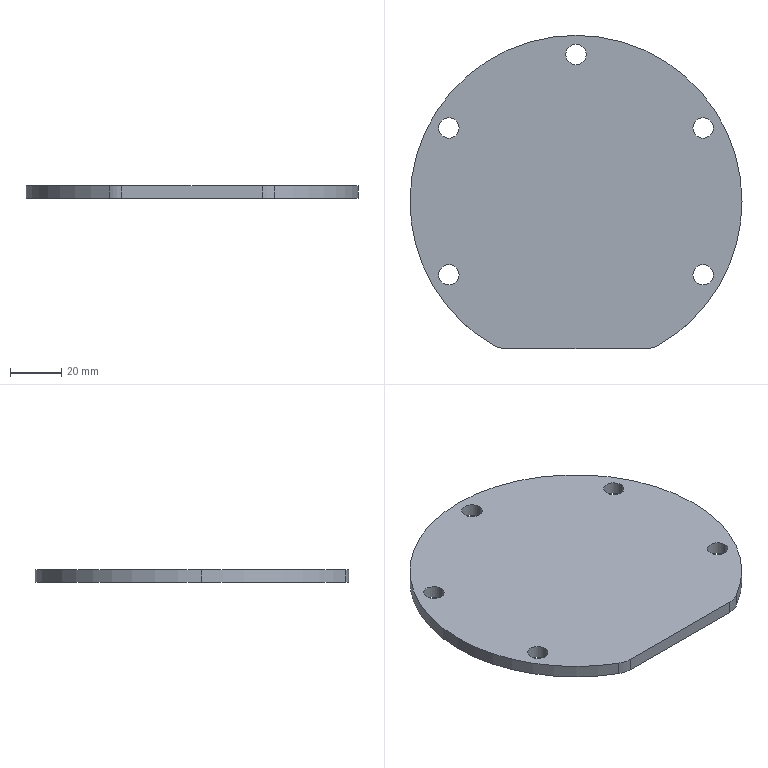Part | STEP file | VD-SYL0380DJ1006_1-3_VD-SYL0380 | 1 solid | 18 faces | box 130 x 122.663 x 5 mm | volume 63619 mm3 | cylinder 15 | plane 3 | commonest cylinder face diameters 8 x10 130 x3 20 x2
STEP:
#1=CARTESIAN_POINT('',(4.,57.5,0.));
#2=VERTEX_POINT('',#1);
#3=CARTESIAN_POINT('',(-4.,57.5,0.));
#4=VERTEX_POINT('',#3);
#5=CARTESIAN_POINT('',(0.,57.5,0.));
#6=DIRECTION('',(0.,0.,1.));
#7=DIRECTION('',(1.,0.,0.));
#8=AXIS2_PLACEMENT_3D('',#5,#6,#7);
#9=CIRCLE('',#8,4.);
#10=EDGE_CURVE('',#2,#4,#9,.T.);
#11=ORIENTED_EDGE('',*,*,#10,.F.);
#12=CARTESIAN_POINT('',(4.,57.5,5.));
#13=VERTEX_POINT('',#12);
#14=CARTESIAN_POINT('',(4.,57.5,5.));
#15=DIRECTION('',(0.,0.,-1.));
#16=VECTOR('',#15,1000.);
#17=LINE('',#14,#16);
#18=EDGE_CURVE('',#13,#2,#17,.T.);
#19=ORIENTED_EDGE('',*,*,#18,.F.);
#20=CARTESIAN_POINT('',(-4.,57.5,5.));
#21=VERTEX_POINT('',#20);
#22=CARTESIAN_POINT('',(0.,57.5,5.));
#23=DIRECTION('',(0.,0.,-1.));
#24=DIRECTION('',(-1.,0.,0.));
#25=AXIS2_PLACEMENT_3D('',#22,#23,#24);
#26=CIRCLE('',#25,4.);
#27=EDGE_CURVE('',#21,#13,#26,.T.);
#28=ORIENTED_EDGE('',*,*,#27,.F.);
#29=CARTESIAN_POINT('',(-4.,57.5,5.));
#30=DIRECTION('',(0.,0.,-1.));
#31=VECTOR('',#30,1000.);
#32=LINE('',#29,#31);
#33=EDGE_CURVE('',#21,#4,#32,.T.);
#34=ORIENTED_EDGE('',*,*,#33,.T.);
#35=EDGE_LOOP('',(#11,#19,#28,#34));
#36=FACE_OUTER_BOUND('',#35,.T.);
#37=CARTESIAN_POINT('',(0.,57.5,2.5));
#38=DIRECTION('',(0.,0.,1.));
#39=DIRECTION('',(1.,0.,0.));
#40=AXIS2_PLACEMENT_3D('',#37,#38,#39);
#41=CYLINDRICAL_SURFACE('',#40,4.);
#42=ADVANCED_FACE('',(#36),#41,.F.);
#43=ORIENTED_EDGE('',*,*,#33,.F.);
#44=CARTESIAN_POINT('',(0.,57.5,5.));
#45=DIRECTION('',(0.,0.,-1.));
#46=DIRECTION('',(1.,0.,0.));
#47=AXIS2_PLACEMENT_3D('',#44,#45,#46);
#48=CIRCLE('',#47,4.);
#49=EDGE_CURVE('',#13,#21,#48,.T.);
#50=ORIENTED_EDGE('',*,*,#49,.F.);
#51=ORIENTED_EDGE('',*,*,#18,.T.);
#52=CARTESIAN_POINT('',(0.,57.5,0.));
#53=DIRECTION('',(0.,0.,1.));
#54=DIRECTION('',(-1.,0.,0.));
#55=AXIS2_PLACEMENT_3D('',#52,#53,#54);
#56=CIRCLE('',#55,4.);
#57=EDGE_CURVE('',#4,#2,#56,.T.);
#58=ORIENTED_EDGE('',*,*,#57,.F.);
#59=EDGE_LOOP('',(#43,#50,#51,#58));
#60=FACE_OUTER_BOUND('',#59,.T.);
#61=CARTESIAN_POINT('',(0.,57.5,2.5));
#62=DIRECTION('',(0.,0.,1.));
#63=DIRECTION('',(1.,0.,0.));
#64=AXIS2_PLACEMENT_3D('',#61,#62,#63);
#65=CYLINDRICAL_SURFACE('',#64,4.);
#66=ADVANCED_FACE('',(#60),#65,.F.);
#67=CARTESIAN_POINT('',(-45.796,28.75,0.));
#68=VERTEX_POINT('',#67);
#69=CARTESIAN_POINT('',(-53.796,28.75,0.));
#70=VERTEX_POINT('',#69);
#71=CARTESIAN_POINT('',(-49.796,28.75,0.));
#72=DIRECTION('',(0.,0.,1.));
#73=DIRECTION('',(1.,0.,0.));
#74=AXIS2_PLACEMENT_3D('',#71,#72,#73);
#75=CIRCLE('',#74,4.);
#76=EDGE_CURVE('',#68,#70,#75,.T.);
#77=ORIENTED_EDGE('',*,*,#76,.F.);
#78=CARTESIAN_POINT('',(-45.796,28.75,5.));
#79=VERTEX_POINT('',#78);
#80=CARTESIAN_POINT('',(-45.796,28.75,5.));
#81=DIRECTION('',(0.,0.,-1.));
#82=VECTOR('',#81,1000.);
#83=LINE('',#80,#82);
#84=EDGE_CURVE('',#79,#68,#83,.T.);
#85=ORIENTED_EDGE('',*,*,#84,.F.);
#86=CARTESIAN_POINT('',(-53.796,28.75,5.));
#87=VERTEX_POINT('',#86);
#88=CARTESIAN_POINT('',(-49.796,28.75,5.));
#89=DIRECTION('',(0.,0.,-1.));
#90=DIRECTION('',(-1.,0.,0.));
#91=AXIS2_PLACEMENT_3D('',#88,#89,#90);
#92=CIRCLE('',#91,4.);
#93=EDGE_CURVE('',#87,#79,#92,.T.);
#94=ORIENTED_EDGE('',*,*,#93,.F.);
#95=CARTESIAN_POINT('',(-53.796,28.75,5.));
#96=DIRECTION('',(0.,0.,-1.));
#97=VECTOR('',#96,1000.);
#98=LINE('',#95,#97);
#99=EDGE_CURVE('',#87,#70,#98,.T.);
#100=ORIENTED_EDGE('',*,*,#99,.T.);
#101=EDGE_LOOP('',(#77,#85,#94,#100));
#102=FACE_OUTER_BOUND('',#101,.T.);
#103=CARTESIAN_POINT('',(-49.796,28.75,2.5));
#104=DIRECTION('',(0.,0.,1.));
#105=DIRECTION('',(1.,0.,0.));
#106=AXIS2_PLACEMENT_3D('',#103,#104,#105);
#107=CYLINDRICAL_SURFACE('',#106,4.);
#108=ADVANCED_FACE('',(#102),#107,.F.);
#109=ORIENTED_EDGE('',*,*,#99,.F.);
#110=CARTESIAN_POINT('',(-49.796,28.75,5.));
#111=DIRECTION('',(0.,0.,-1.));
#112=DIRECTION('',(1.,0.,0.));
#113=AXIS2_PLACEMENT_3D('',#110,#111,#112);
#114=CIRCLE('',#113,4.);
#115=EDGE_CURVE('',#79,#87,#114,.T.);
#116=ORIENTED_EDGE('',*,*,#115,.F.);
#117=ORIENTED_EDGE('',*,*,#84,.T.);
#118=CARTESIAN_POINT('',(-49.796,28.75,0.));
#119=DIRECTION('',(0.,0.,1.));
#120=DIRECTION('',(-1.,0.,0.));
#121=AXIS2_PLACEMENT_3D('',#118,#119,#120);
#122=CIRCLE('',#121,4.);
#123=EDGE_CURVE('',#70,#68,#122,.T.);
#124=ORIENTED_EDGE('',*,*,#123,.F.);
#125=EDGE_LOOP('',(#109,#116,#117,#124));
#126=FACE_OUTER_BOUND('',#125,.T.);
#127=CARTESIAN_POINT('',(-49.796,28.75,2.5));
#128=DIRECTION('',(0.,0.,1.));
#129=DIRECTION('',(1.,0.,0.));
#130=AXIS2_PLACEMENT_3D('',#127,#128,#129);
#131=CYLINDRICAL_SURFACE('',#130,4.);
#132=ADVANCED_FACE('',(#126),#131,.F.);
#133=CARTESIAN_POINT('',(-45.796,-28.75,0.));
#134=VERTEX_POINT('',#133);
#135=CARTESIAN_POINT('',(-53.796,-28.75,0.));
#136=VERTEX_POINT('',#135);
#137=CARTESIAN_POINT('',(-49.796,-28.75,0.));
#138=DIRECTION('',(0.,0.,1.));
#139=DIRECTION('',(1.,0.,0.));
#140=AXIS2_PLACEMENT_3D('',#137,#138,#139);
#141=CIRCLE('',#140,4.);
#142=EDGE_CURVE('',#134,#136,#141,.T.);
#143=ORIENTED_EDGE('',*,*,#142,.F.);
#144=CARTESIAN_POINT('',(-45.796,-28.75,5.));
#145=VERTEX_POINT('',#144);
#146=CARTESIAN_POINT('',(-45.796,-28.75,5.));
#147=DIRECTION('',(0.,0.,-1.));
#148=VECTOR('',#147,1000.);
#149=LINE('',#146,#148);
#150=EDGE_CURVE('',#145,#134,#149,.T.);
#151=ORIENTED_EDGE('',*,*,#150,.F.);
#152=CARTESIAN_POINT('',(-53.796,-28.75,5.));
#153=VERTEX_POINT('',#152);
#154=CARTESIAN_POINT('',(-49.796,-28.75,5.));
#155=DIRECTION('',(0.,0.,-1.));
#156=DIRECTION('',(-1.,0.,0.));
#157=AXIS2_PLACEMENT_3D('',#154,#155,#156);
#158=CIRCLE('',#157,4.);
#159=EDGE_CURVE('',#153,#145,#158,.T.);
#160=ORIENTED_EDGE('',*,*,#159,.F.);
#161=CARTESIAN_POINT('',(-53.796,-28.75,5.));
#162=DIRECTION('',(0.,0.,-1.));
#163=VECTOR('',#162,1000.);
#164=LINE('',#161,#163);
#165=EDGE_CURVE('',#153,#136,#164,.T.);
#166=ORIENTED_EDGE('',*,*,#165,.T.);
#167=EDGE_LOOP('',(#143,#151,#160,#166));
#168=FACE_OUTER_BOUND('',#167,.T.);
#169=CARTESIAN_POINT('',(-49.796,-28.75,2.5));
#170=DIRECTION('',(0.,0.,1.));
#171=DIRECTION('',(1.,0.,0.));
#172=AXIS2_PLACEMENT_3D('',#169,#170,#171);
#173=CYLINDRICAL_SURFACE('',#172,4.);
#174=ADVANCED_FACE('',(#168),#173,.F.);
#175=ORIENTED_EDGE('',*,*,#165,.F.);
#176=CARTESIAN_POINT('',(-49.796,-28.75,5.));
#177=DIRECTION('',(0.,0.,-1.));
#178=DIRECTION('',(1.,0.,0.));
#179=AXIS2_PLACEMENT_3D('',#176,#177,#178);
#180=CIRCLE('',#179,4.);
#181=EDGE_CURVE('',#145,#153,#180,.T.);
#182=ORIENTED_EDGE('',*,*,#181,.F.);
#183=ORIENTED_EDGE('',*,*,#150,.T.);
#184=CARTESIAN_POINT('',(-49.796,-28.75,0.));
#185=DIRECTION('',(0.,0.,1.));
#186=DIRECTION('',(-1.,0.,0.));
#187=AXIS2_PLACEMENT_3D('',#184,#185,#186);
#188=CIRCLE('',#187,4.);
#189=EDGE_CURVE('',#136,#134,#188,.T.);
#190=ORIENTED_EDGE('',*,*,#189,.F.);
#191=EDGE_LOOP('',(#175,#182,#183,#190));
#192=FACE_OUTER_BOUND('',#191,.T.);
#193=CARTESIAN_POINT('',(-49.796,-28.75,2.5));
#194=DIRECTION('',(0.,0.,1.));
#195=DIRECTION('',(1.,0.,0.));
#196=AXIS2_PLACEMENT_3D('',#193,#194,#195);
#197=CYLINDRICAL_SURFACE('',#196,4.);
#198=ADVANCED_FACE('',(#192),#197,.F.);
#199=CARTESIAN_POINT('',(53.796,-28.75,0.));
#200=VERTEX_POINT('',#199);
#201=CARTESIAN_POINT('',(45.796,-28.75,0.));
#202=VERTEX_POINT('',#201);
#203=CARTESIAN_POINT('',(49.796,-28.75,0.));
#204=DIRECTION('',(0.,0.,1.));
#205=DIRECTION('',(1.,0.,0.));
#206=AXIS2_PLACEMENT_3D('',#203,#204,#205);
#207=CIRCLE('',#206,4.);
#208=EDGE_CURVE('',#200,#202,#207,.T.);
#209=ORIENTED_EDGE('',*,*,#208,.F.);
#210=CARTESIAN_POINT('',(53.796,-28.75,5.));
#211=VERTEX_POINT('',#210);
#212=CARTESIAN_POINT('',(53.796,-28.75,5.));
#213=DIRECTION('',(0.,0.,-1.));
#214=VECTOR('',#213,1000.);
#215=LINE('',#212,#214);
#216=EDGE_CURVE('',#211,#200,#215,.T.);
#217=ORIENTED_EDGE('',*,*,#216,.F.);
#218=CARTESIAN_POINT('',(45.796,-28.75,5.));
#219=VERTEX_POINT('',#218);
#220=CARTESIAN_POINT('',(49.796,-28.75,5.));
#221=DIRECTION('',(0.,0.,-1.));
#222=DIRECTION('',(-1.,0.,0.));
#223=AXIS2_PLACEMENT_3D('',#220,#221,#222);
#224=CIRCLE('',#223,4.);
#225=EDGE_CURVE('',#219,#211,#224,.T.);
#226=ORIENTED_EDGE('',*,*,#225,.F.);
#227=CARTESIAN_POINT('',(45.796,-28.75,5.));
#228=DIRECTION('',(0.,0.,-1.));
#229=VECTOR('',#228,1000.);
#230=LINE('',#227,#229);
#231=EDGE_CURVE('',#219,#202,#230,.T.);
#232=ORIENTED_EDGE('',*,*,#231,.T.);
#233=EDGE_LOOP('',(#209,#217,#226,#232));
#234=FACE_OUTER_BOUND('',#233,.T.);
#235=CARTESIAN_POINT('',(49.796,-28.75,2.5));
#236=DIRECTION('',(0.,0.,1.));
#237=DIRECTION('',(1.,0.,0.));
#238=AXIS2_PLACEMENT_3D('',#235,#236,#237);
#239=CYLINDRICAL_SURFACE('',#238,4.);
#240=ADVANCED_FACE('',(#234),#239,.F.);
#241=ORIENTED_EDGE('',*,*,#231,.F.);
#242=CARTESIAN_POINT('',(49.796,-28.75,5.));
#243=DIRECTION('',(0.,0.,-1.));
#244=DIRECTION('',(1.,0.,0.));
#245=AXIS2_PLACEMENT_3D('',#242,#243,#244);
#246=CIRCLE('',#245,4.);
#247=EDGE_CURVE('',#211,#219,#246,.T.);
#248=ORIENTED_EDGE('',*,*,#247,.F.);
#249=ORIENTED_EDGE('',*,*,#216,.T.);
#250=CARTESIAN_POINT('',(49.796,-28.75,0.));
#251=DIRECTION('',(0.,0.,1.));
#252=DIRECTION('',(-1.,0.,0.));
#253=AXIS2_PLACEMENT_3D('',#250,#251,#252);
#254=CIRCLE('',#253,4.);
#255=EDGE_CURVE('',#202,#200,#254,.T.);
#256=ORIENTED_EDGE('',*,*,#255,.F.);
#257=EDGE_LOOP('',(#241,#248,#249,#256));
#258=FACE_OUTER_BOUND('',#257,.T.);
#259=CARTESIAN_POINT('',(49.796,-28.75,2.5));
#260=DIRECTION('',(0.,0.,1.));
#261=DIRECTION('',(1.,0.,0.));
#262=AXIS2_PLACEMENT_3D('',#259,#260,#261);
#263=CYLINDRICAL_SURFACE('',#262,4.);
#264=ADVANCED_FACE('',(#258),#263,.F.);
#265=CARTESIAN_POINT('',(53.796,28.75,0.));
#266=VERTEX_POINT('',#265);
#267=CARTESIAN_POINT('',(45.796,28.75,0.));
#268=VERTEX_POINT('',#267);
#269=CARTESIAN_POINT('',(49.796,28.75,0.));
#270=DIRECTION('',(0.,0.,1.));
#271=DIRECTION('',(1.,0.,0.));
#272=AXIS2_PLACEMENT_3D('',#269,#270,#271);
#273=CIRCLE('',#272,4.);
#274=EDGE_CURVE('',#266,#268,#273,.T.);
#275=ORIENTED_EDGE('',*,*,#274,.F.);
#276=CARTESIAN_POINT('',(53.796,28.75,5.));
#277=VERTEX_POINT('',#276);
#278=CARTESIAN_POINT('',(53.796,28.75,5.));
#279=DIRECTION('',(0.,0.,-1.));
#280=VECTOR('',#279,1000.);
#281=LINE('',#278,#280);
#282=EDGE_CURVE('',#277,#266,#281,.T.);
#283=ORIENTED_EDGE('',*,*,#282,.F.);
#284=CARTESIAN_POINT('',(45.796,28.75,5.));
#285=VERTEX_POINT('',#284);
#286=CARTESIAN_POINT('',(49.796,28.75,5.));
#287=DIRECTION('',(0.,0.,-1.));
#288=DIRECTION('',(-1.,0.,0.));
#289=AXIS2_PLACEMENT_3D('',#286,#287,#288);
#290=CIRCLE('',#289,4.);
#291=EDGE_CURVE('',#285,#277,#290,.T.);
#292=ORIENTED_EDGE('',*,*,#291,.F.);
#293=CARTESIAN_POINT('',(45.796,28.75,5.));
#294=DIRECTION('',(0.,0.,-1.));
#295=VECTOR('',#294,1000.);
#296=LINE('',#293,#295);
#297=EDGE_CURVE('',#285,#268,#296,.T.);
#298=ORIENTED_EDGE('',*,*,#297,.T.);
#299=EDGE_LOOP('',(#275,#283,#292,#298));
#300=FACE_OUTER_BOUND('',#299,.T.);
#301=CARTESIAN_POINT('',(49.796,28.75,2.5));
#302=DIRECTION('',(0.,0.,1.));
#303=DIRECTION('',(1.,0.,0.));
#304=AXIS2_PLACEMENT_3D('',#301,#302,#303);
#305=CYLINDRICAL_SURFACE('',#304,4.);
#306=ADVANCED_FACE('',(#300),#305,.F.);
#307=ORIENTED_EDGE('',*,*,#297,.F.);
#308=CARTESIAN_POINT('',(49.796,28.75,5.));
#309=DIRECTION('',(0.,0.,-1.));
#310=DIRECTION('',(1.,0.,0.));
#311=AXIS2_PLACEMENT_3D('',#308,#309,#310);
#312=CIRCLE('',#311,4.);
#313=EDGE_CURVE('',#277,#285,#312,.T.);
#314=ORIENTED_EDGE('',*,*,#313,.F.);
#315=ORIENTED_EDGE('',*,*,#282,.T.);
#316=CARTESIAN_POINT('',(49.796,28.75,0.));
#317=DIRECTION('',(0.,0.,1.));
#318=DIRECTION('',(-1.,0.,0.));
#319=AXIS2_PLACEMENT_3D('',#316,#317,#318);
#320=CIRCLE('',#319,4.);
#321=EDGE_CURVE('',#268,#266,#320,.T.);
#322=ORIENTED_EDGE('',*,*,#321,.F.);
#323=EDGE_LOOP('',(#307,#314,#315,#322));
#324=FACE_OUTER_BOUND('',#323,.T.);
#325=CARTESIAN_POINT('',(49.796,28.75,2.5));
#326=DIRECTION('',(0.,0.,1.));
#327=DIRECTION('',(1.,0.,0.));
#328=AXIS2_PLACEMENT_3D('',#325,#326,#327);
#329=CYLINDRICAL_SURFACE('',#328,4.);
#330=ADVANCED_FACE('',(#324),#329,.F.);
#331=CARTESIAN_POINT('',(-27.446,-57.663,0.));
#332=VERTEX_POINT('',#331);
#333=CARTESIAN_POINT('',(-32.436,-56.329,0.));
#334=VERTEX_POINT('',#333);
#335=CARTESIAN_POINT('',(-27.446,-47.663,0.));
#336=DIRECTION('',(0.,0.,-1.));
#337=DIRECTION('',(0.,-1.,0.));
#338=AXIS2_PLACEMENT_3D('',#335,#336,#337);
#339=CIRCLE('',#338,10.);
#340=EDGE_CURVE('',#332,#334,#339,.T.);
#341=ORIENTED_EDGE('',*,*,#340,.F.);
#342=CARTESIAN_POINT('',(-27.446,-57.663,5.));
#343=VERTEX_POINT('',#342);
#344=CARTESIAN_POINT('',(-27.446,-57.663,0.));
#345=DIRECTION('',(0.,0.,1.));
#346=VECTOR('',#345,1000.);
#347=LINE('',#344,#346);
#348=EDGE_CURVE('',#332,#343,#347,.T.);
#349=ORIENTED_EDGE('',*,*,#348,.T.);
#350=CARTESIAN_POINT('',(-32.436,-56.329,5.));
#351=VERTEX_POINT('',#350);
#352=CARTESIAN_POINT('',(-27.446,-47.663,5.));
#353=DIRECTION('',(0.,0.,1.));
#354=DIRECTION('',(-0.499,-0.8666,0.));
#355=AXIS2_PLACEMENT_3D('',#352,#353,#354);
#356=CIRCLE('',#355,10.);
#357=EDGE_CURVE('',#351,#343,#356,.T.);
#358=ORIENTED_EDGE('',*,*,#357,.F.);
#359=CARTESIAN_POINT('',(-32.436,-56.329,5.));
#360=DIRECTION('',(0.,0.,-1.));
#361=VECTOR('',#360,1000.);
#362=LINE('',#359,#361);
#363=EDGE_CURVE('',#351,#334,#362,.T.);
#364=ORIENTED_EDGE('',*,*,#363,.T.);
#365=EDGE_LOOP('',(#341,#349,#358,#364));
#366=FACE_OUTER_BOUND('',#365,.T.);
#367=CARTESIAN_POINT('',(-27.446,-47.663,17.53));
#368=DIRECTION('',(0.,0.,-1.));
#369=DIRECTION('',(-1.,0.,0.));
#370=AXIS2_PLACEMENT_3D('',#367,#368,#369);
#371=CYLINDRICAL_SURFACE('',#370,10.);
#372=ADVANCED_FACE('',(#366),#371,.T.);
#373=CARTESIAN_POINT('',(65.,0.,5.));
#374=VERTEX_POINT('',#373);
#375=CARTESIAN_POINT('',(65.,0.,0.));
#376=VERTEX_POINT('',#375);
#377=CARTESIAN_POINT('',(65.,0.,5.));
#378=DIRECTION('',(0.,0.,-1.));
#379=VECTOR('',#378,1000.);
#380=LINE('',#377,#379);
#381=EDGE_CURVE('',#374,#376,#380,.T.);
#382=ORIENTED_EDGE('',*,*,#381,.F.);
#383=CARTESIAN_POINT('',(32.436,-56.329,5.));
#384=VERTEX_POINT('',#383);
#385=CARTESIAN_POINT('',(0.,0.,5.));
#386=DIRECTION('',(0.,0.,1.));
#387=DIRECTION('',(0.499,-0.8666,0.));
#388=AXIS2_PLACEMENT_3D('',#385,#386,#387);
#389=CIRCLE('',#388,65.);
#390=EDGE_CURVE('',#384,#374,#389,.T.);
#391=ORIENTED_EDGE('',*,*,#390,.F.);
#392=CARTESIAN_POINT('',(32.436,-56.329,0.));
#393=VERTEX_POINT('',#392);
#394=CARTESIAN_POINT('',(32.436,-56.329,0.));
#395=DIRECTION('',(0.,0.,1.));
#396=VECTOR('',#395,1000.);
#397=LINE('',#394,#396);
#398=EDGE_CURVE('',#393,#384,#397,.T.);
#399=ORIENTED_EDGE('',*,*,#398,.F.);
#400=CARTESIAN_POINT('',(0.,0.,0.));
#401=DIRECTION('',(0.,0.,-1.));
#402=DIRECTION('',(1.,0.,0.));
#403=AXIS2_PLACEMENT_3D('',#400,#401,#402);
#404=CIRCLE('',#403,65.);
#405=EDGE_CURVE('',#376,#393,#404,.T.);
#406=ORIENTED_EDGE('',*,*,#405,.F.);
#407=EDGE_LOOP('',(#382,#391,#399,#406));
#408=FACE_OUTER_BOUND('',#407,.T.);
#409=CARTESIAN_POINT('',(0.,0.,2.5));
#410=DIRECTION('',(0.,0.,1.));
#411=DIRECTION('',(1.,0.,0.));
#412=AXIS2_PLACEMENT_3D('',#409,#410,#411);
#413=CYLINDRICAL_SURFACE('',#412,65.);
#414=ADVANCED_FACE('',(#408),#413,.T.);
#415=ORIENTED_EDGE('',*,*,#10,.T.);
#416=ORIENTED_EDGE('',*,*,#57,.T.);
#417=EDGE_LOOP('',(#415,#416));
#418=FACE_BOUND('',#417,.T.);
#419=ORIENTED_EDGE('',*,*,#76,.T.);
#420=ORIENTED_EDGE('',*,*,#123,.T.);
#421=EDGE_LOOP('',(#419,#420));
#422=FACE_BOUND('',#421,.T.);
#423=ORIENTED_EDGE('',*,*,#142,.T.);
#424=ORIENTED_EDGE('',*,*,#189,.T.);
#425=EDGE_LOOP('',(#423,#424));
#426=FACE_BOUND('',#425,.T.);
#427=ORIENTED_EDGE('',*,*,#208,.T.);
#428=ORIENTED_EDGE('',*,*,#255,.T.);
#429=EDGE_LOOP('',(#427,#428));
#430=FACE_BOUND('',#429,.T.);
#431=ORIENTED_EDGE('',*,*,#274,.T.);
#432=ORIENTED_EDGE('',*,*,#321,.T.);
#433=EDGE_LOOP('',(#431,#432));
#434=FACE_BOUND('',#433,.T.);
#435=CARTESIAN_POINT('',(27.446,-57.663,0.));
#436=VERTEX_POINT('',#435);
#437=CARTESIAN_POINT('',(27.446,-57.663,0.));
#438=DIRECTION('',(-1.,0.,0.));
#439=VECTOR('',#438,1000.);
#440=LINE('',#437,#439);
#441=EDGE_CURVE('',#436,#332,#440,.T.);
#442=ORIENTED_EDGE('',*,*,#441,.T.);
#443=ORIENTED_EDGE('',*,*,#340,.T.);
#444=CARTESIAN_POINT('',(-65.,0.,0.));
#445=VERTEX_POINT('',#444);
#446=CARTESIAN_POINT('',(0.,0.,0.));
#447=DIRECTION('',(0.,0.,-1.));
#448=DIRECTION('',(-0.499,-0.8666,0.));
#449=AXIS2_PLACEMENT_3D('',#446,#447,#448);
#450=CIRCLE('',#449,65.);
#451=EDGE_CURVE('',#334,#445,#450,.T.);
#452=ORIENTED_EDGE('',*,*,#451,.T.);
#453=CARTESIAN_POINT('',(0.,0.,0.));
#454=DIRECTION('',(0.,0.,-1.));
#455=DIRECTION('',(-1.,0.,0.));
#456=AXIS2_PLACEMENT_3D('',#453,#454,#455);
#457=CIRCLE('',#456,65.);
#458=EDGE_CURVE('',#445,#376,#457,.T.);
#459=ORIENTED_EDGE('',*,*,#458,.T.);
#460=ORIENTED_EDGE('',*,*,#405,.T.);
#461=CARTESIAN_POINT('',(27.446,-47.663,0.));
#462=DIRECTION('',(0.,0.,-1.));
#463=DIRECTION('',(0.499,-0.8666,0.));
#464=AXIS2_PLACEMENT_3D('',#461,#462,#463);
#465=CIRCLE('',#464,10.);
#466=EDGE_CURVE('',#393,#436,#465,.T.);
#467=ORIENTED_EDGE('',*,*,#466,.T.);
#468=EDGE_LOOP('',(#442,#443,#452,#459,#460,#467));
#469=FACE_OUTER_BOUND('',#468,.T.);
#470=CARTESIAN_POINT('',(0.,0.,0.));
#471=DIRECTION('',(0.,0.,1.));
#472=DIRECTION('',(1.,0.,0.));
#473=AXIS2_PLACEMENT_3D('',#470,#471,#472);
#474=PLANE('',#473);
#475=ADVANCED_FACE('',(#418,#422,#426,#430,#434,#469),#474,.F.);
#476=CARTESIAN_POINT('',(-65.,0.,5.));
#477=VERTEX_POINT('',#476);
#478=CARTESIAN_POINT('',(-65.,0.,5.));
#479=DIRECTION('',(0.,0.,-1.));
#480=VECTOR('',#479,1000.);
#481=LINE('',#478,#480);
#482=EDGE_CURVE('',#477,#445,#481,.T.);
#483=ORIENTED_EDGE('',*,*,#482,.F.);
#484=CARTESIAN_POINT('',(0.,0.,5.));
#485=DIRECTION('',(0.,0.,1.));
#486=DIRECTION('',(1.,0.,0.));
#487=AXIS2_PLACEMENT_3D('',#484,#485,#486);
#488=CIRCLE('',#487,65.);
#489=EDGE_CURVE('',#374,#477,#488,.T.);
#490=ORIENTED_EDGE('',*,*,#489,.F.);
#491=ORIENTED_EDGE('',*,*,#381,.T.);
#492=ORIENTED_EDGE('',*,*,#458,.F.);
#493=EDGE_LOOP('',(#483,#490,#491,#492));
#494=FACE_OUTER_BOUND('',#493,.T.);
#495=CARTESIAN_POINT('',(0.,0.,2.5));
#496=DIRECTION('',(0.,0.,1.));
#497=DIRECTION('',(1.,0.,0.));
#498=AXIS2_PLACEMENT_3D('',#495,#496,#497);
#499=CYLINDRICAL_SURFACE('',#498,65.);
#500=ADVANCED_FACE('',(#494),#499,.T.);
#501=ORIENTED_EDGE('',*,*,#451,.F.);
#502=ORIENTED_EDGE('',*,*,#363,.F.);
#503=CARTESIAN_POINT('',(0.,0.,5.));
#504=DIRECTION('',(0.,0.,1.));
#505=DIRECTION('',(-1.,0.,0.));
#506=AXIS2_PLACEMENT_3D('',#503,#504,#505);
#507=CIRCLE('',#506,65.);
#508=EDGE_CURVE('',#477,#351,#507,.T.);
#509=ORIENTED_EDGE('',*,*,#508,.F.);
#510=ORIENTED_EDGE('',*,*,#482,.T.);
#511=EDGE_LOOP('',(#501,#502,#509,#510));
#512=FACE_OUTER_BOUND('',#511,.T.);
#513=CARTESIAN_POINT('',(0.,0.,2.5));
#514=DIRECTION('',(0.,0.,1.));
#515=DIRECTION('',(1.,0.,0.));
#516=AXIS2_PLACEMENT_3D('',#513,#514,#515);
#517=CYLINDRICAL_SURFACE('',#516,65.);
#518=ADVANCED_FACE('',(#512),#517,.T.);
#519=ORIENTED_EDGE('',*,*,#27,.T.);
#520=ORIENTED_EDGE('',*,*,#49,.T.);
#521=EDGE_LOOP('',(#519,#520));
#522=FACE_BOUND('',#521,.T.);
#523=ORIENTED_EDGE('',*,*,#93,.T.);
#524=ORIENTED_EDGE('',*,*,#115,.T.);
#525=EDGE_LOOP('',(#523,#524));
#526=FACE_BOUND('',#525,.T.);
#527=ORIENTED_EDGE('',*,*,#159,.T.);
#528=ORIENTED_EDGE('',*,*,#181,.T.);
#529=EDGE_LOOP('',(#527,#528));
#530=FACE_BOUND('',#529,.T.);
#531=ORIENTED_EDGE('',*,*,#225,.T.);
#532=ORIENTED_EDGE('',*,*,#247,.T.);
#533=EDGE_LOOP('',(#531,#532));
#534=FACE_BOUND('',#533,.T.);
#535=ORIENTED_EDGE('',*,*,#291,.T.);
#536=ORIENTED_EDGE('',*,*,#313,.T.);
#537=EDGE_LOOP('',(#535,#536));
#538=FACE_BOUND('',#537,.T.);
#539=ORIENTED_EDGE('',*,*,#357,.T.);
#540=CARTESIAN_POINT('',(27.446,-57.663,5.));
#541=VERTEX_POINT('',#540);
#542=CARTESIAN_POINT('',(27.446,-57.663,5.));
#543=DIRECTION('',(-1.,0.,0.));
#544=VECTOR('',#543,1000.);
#545=LINE('',#542,#544);
#546=EDGE_CURVE('',#541,#343,#545,.T.);
#547=ORIENTED_EDGE('',*,*,#546,.F.);
#548=CARTESIAN_POINT('',(27.446,-47.663,5.));
#549=DIRECTION('',(0.,0.,1.));
#550=DIRECTION('',(0.,-1.,0.));
#551=AXIS2_PLACEMENT_3D('',#548,#549,#550);
#552=CIRCLE('',#551,10.);
#553=EDGE_CURVE('',#541,#384,#552,.T.);
#554=ORIENTED_EDGE('',*,*,#553,.T.);
#555=ORIENTED_EDGE('',*,*,#390,.T.);
#556=ORIENTED_EDGE('',*,*,#489,.T.);
#557=ORIENTED_EDGE('',*,*,#508,.T.);
#558=EDGE_LOOP('',(#539,#547,#554,#555,#556,#557));
#559=FACE_OUTER_BOUND('',#558,.T.);
#560=CARTESIAN_POINT('',(0.,0.,5.));
#561=DIRECTION('',(0.,0.,1.));
#562=DIRECTION('',(1.,0.,0.));
#563=AXIS2_PLACEMENT_3D('',#560,#561,#562);
#564=PLANE('',#563);
#565=ADVANCED_FACE('',(#522,#526,#530,#534,#538,#559),#564,.T.);
#566=ORIENTED_EDGE('',*,*,#466,.F.);
#567=ORIENTED_EDGE('',*,*,#398,.T.);
#568=ORIENTED_EDGE('',*,*,#553,.F.);
#569=CARTESIAN_POINT('',(27.446,-57.663,5.));
#570=DIRECTION('',(0.,0.,-1.));
#571=VECTOR('',#570,1000.);
#572=LINE('',#569,#571);
#573=EDGE_CURVE('',#541,#436,#572,.T.);
#574=ORIENTED_EDGE('',*,*,#573,.T.);
#575=EDGE_LOOP('',(#566,#567,#568,#574));
#576=FACE_OUTER_BOUND('',#575,.T.);
#577=CARTESIAN_POINT('',(27.446,-47.663,17.53));
#578=DIRECTION('',(0.,0.,-1.));
#579=DIRECTION('',(-1.,0.,0.));
#580=AXIS2_PLACEMENT_3D('',#577,#578,#579);
#581=CYLINDRICAL_SURFACE('',#580,10.);
#582=ADVANCED_FACE('',(#576),#581,.T.);
#583=ORIENTED_EDGE('',*,*,#546,.T.);
#584=ORIENTED_EDGE('',*,*,#348,.F.);
#585=ORIENTED_EDGE('',*,*,#441,.F.);
#586=ORIENTED_EDGE('',*,*,#573,.F.);
#587=EDGE_LOOP('',(#583,#584,#585,#586));
#588=FACE_OUTER_BOUND('',#587,.T.);
#589=CARTESIAN_POINT('',(0.,-57.663,2.5));
#590=DIRECTION('',(0.,1.,0.));
#591=DIRECTION('',(1.,0.,0.));
#592=AXIS2_PLACEMENT_3D('',#589,#590,#591);
#593=PLANE('',#592);
#594=ADVANCED_FACE('',(#588),#593,.F.);
#595=CLOSED_SHELL('',(#42,#66,#108,#132,#174,#198,#240,#264,#306,#330,#372,#414,#475,#500,#518,#565,#582,#594));
#596=MANIFOLD_SOLID_BREP('',#595);
#597=CARTESIAN_POINT('',(0.,0.,0.));
#598=DIRECTION('',(0.,0.,1.));
#599=DIRECTION('',(1.,0.,0.));
#600=AXIS2_PLACEMENT_3D('',#597,#598,#599);
#601=(LENGTH_UNIT()NAMED_UNIT(*)SI_UNIT(.MILLI.,.METRE.));
#602=UNCERTAINTY_MEASURE_WITH_UNIT(LENGTH_MEASURE(0.00001),#601,'','');
#603=(NAMED_UNIT(*)PLANE_ANGLE_UNIT()SI_UNIT($,.RADIAN.));
#604=(NAMED_UNIT(*)SI_UNIT($,.STERADIAN.)SOLID_ANGLE_UNIT());
#605=(GEOMETRIC_REPRESENTATION_CONTEXT(3)GLOBAL_UNCERTAINTY_ASSIGNED_CONTEXT((#602))GLOBAL_UNIT_ASSIGNED_CONTEXT((#601,#603,#604))REPRESENTATION_CONTEXT('',''));
#606=ADVANCED_BREP_SHAPE_REPRESENTATION('',(#596,#600),#605);